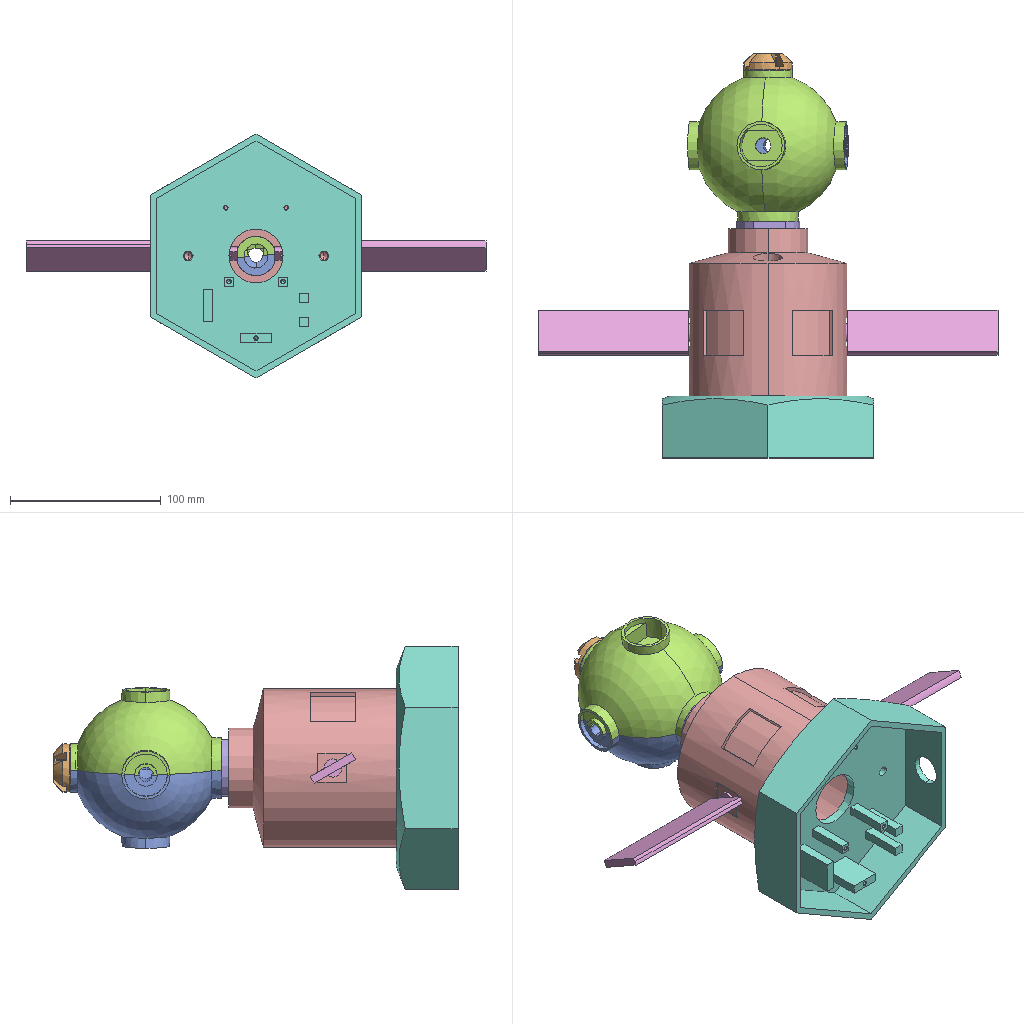Assembly | SolidWorks | 7 different items | 8 placed | box 305 x 268 x 162 mm
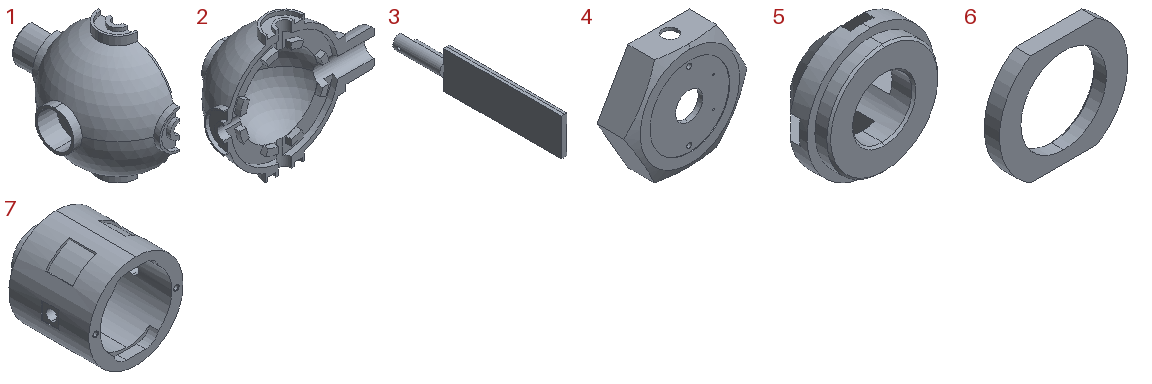Parts list (item | quantity | size | volume | features):
1 | x1 | 56 x 123 x 104 mm | 175814 mm3 | features ICE 15, MirrorPattern 1, RevCut 1, Revolution 1, StudWizard 1
2 | x1 | 123 x 52 x 104 mm | 156554 mm3 | features ICE 15, MirrorPattern 1, RevCut 1, Revolution 1, StudWizard 1
3 | x2 | 12 x 140 x 32 mm | 19807 mm3 | features ICE 3, Extrusion 1, HoleWzd 1
4 | x1 | 161.658 x 41 x 140 mm | 170497 mm3 | features ICE 6, HoleWzd 2, Extrusion 1, RevCut 1
5 | x1 | 32 x 14 x 32 mm | 5204 mm3 | features Chamfer 2, ICE 2, CirPattern 1, Revolution 1
6 | x1 | 42 x 5 x 36 mm | 3362 mm3 | features Extrusion 1, HoleWzd 1
7 | x1 | 105 x 112 x 105 mm | 406446 mm3 | features ICE 5, HoleWzd 2, MirrorPattern 1, RevCut 1, Revolution 1
Mates (type | each side: item.copy, entity, surface, feature):
Coincident | 7.1 plane | assembly plane | 7 times
Concentric | 7.1 face cylinder M30 Tapped Hole1 | 4.1 face cylinder Cut-Extrude3
Coincident | 7.1 face plane Revolve1 | 4.1 face plane Cut-Extrude2
Concentric | 7.1 face cylinder M6 Tapped Hole1 | 4.1 face cylinder Cut-Extrude4
Concentric | 7.1 face cylinder Cut-Extrude4 | 3.1 face cylinder Boss-Extrude1
Tangent | 7.1 face cylinder Revolve1 | 3.1 face plane Cut-Extrude2
Concentric | 1.1 face cylinder Cut-Extrude2 | 2.1 face cylinder Cut-Extrude4
Coincident | 1.1 face plane Revolve1 | 2.1 face plane Revolve1
Concentric | 1.1 face cylinder Boss-Extrude2 | 2.1 face cylinder Boss-Extrude1
Concentric | 7.1 face cylinder M30 Tapped Hole1 | 2.1 face cylinder Boss-Extrude3
Concentric | 2.1 face cylinder Boss-Extrude3 | 6.1 face cylinder M30x2.0 Tapped Hole1
Coincident | 7.1 face plane Revolve1 | 6.1 face plane Boss-Extrude1
Concentric | 2.1 face cylinder Cut-Extrude9 | 5.1 face cylinder Cut-Extrude1
Coincident | 2.1 face plane Cut-Extrude5 | 5.1 face plane Revolve1
Coincident | 1.1 face plane Boss-Extrude3 | 6.1 face plane Boss-Extrude1